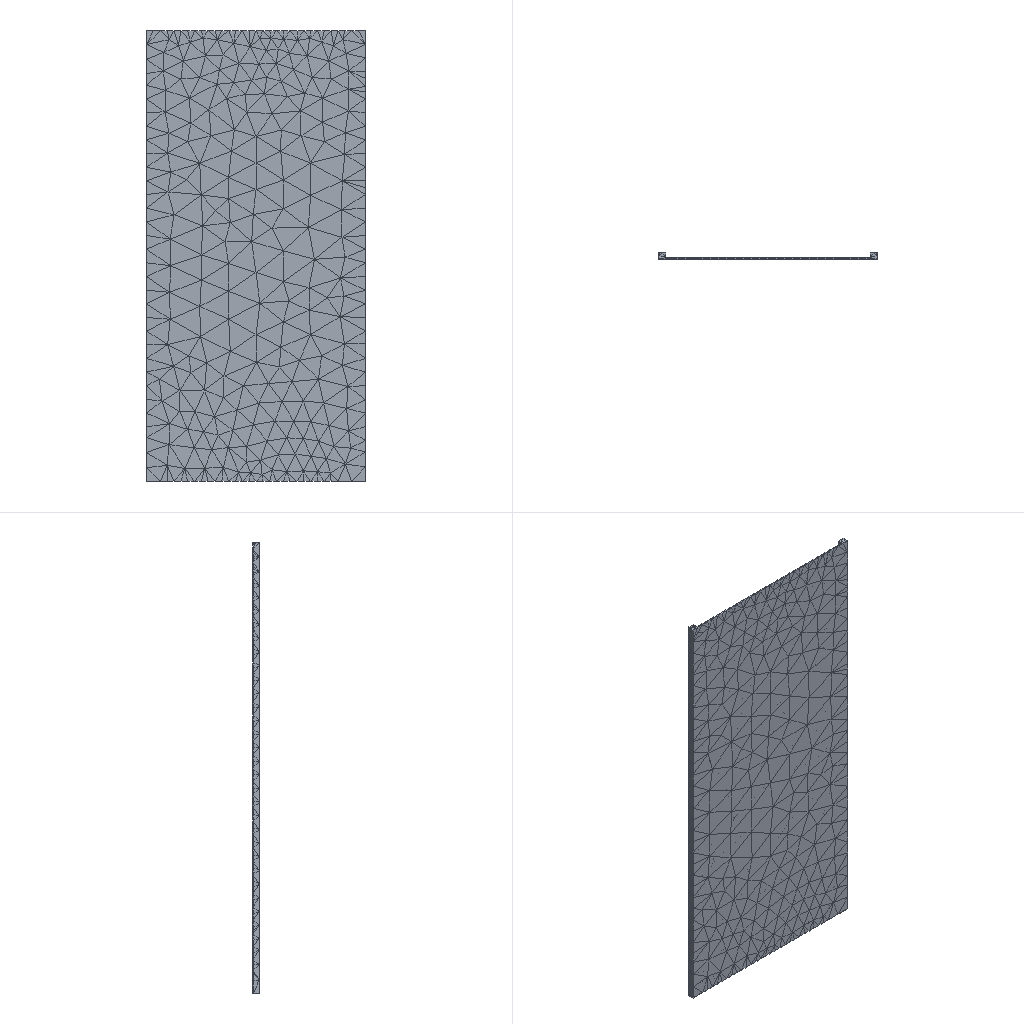Simulation study | ansys workbench
Ansys APDL input file, long lists of numbers shortened:
/batch
/config,noeldb,1     ! force off writing results to database
*get,_wallstrt,active,,time,wall
! ANSYS input file written by Workbench version 2022 R1
! File used for geometry attach: F:\ansys（分析文件汇总)\石材数控线距设备关键零部件分析\Master Assembly.STEP
/title,wbnew--____ (B5)
! ****** Begin Custom Load Command Snippet ******
/COM, ACT Extensions:
/COM,     LSDYNA, 2021.1
/COM,
! ****** End   Custom Load Command Snippet ******
*DIM,_wb_ProjectScratch_dir,string,248
_wb_ProjectScratch_dir(1) = 'C:\Users\Administrator\AppData\Local\Temp\WB_Administrator_1940_2\_ProjectScratch\Scr2DEB\'
*DIM,_wb_SolverFiles_dir,string,248
_wb_SolverFiles_dir(1) = 'C:\Users\Administrator\AppData\Local\Temp\WB_Administrator_1940_2\wbnew_files\dp0\SYS\MECH\'
*DIM,_wb_userfiles_dir,string,248
_wb_userfiles_dir(1) = 'C:\Users\Administrator\AppData\Local\Temp\WB_Administrator_1940_2\wbnew_files\user_files\'
/com,--- Data in consistent NMM units. See Solving Units in the help system for more information.
/units,MPA
/nopr
/wb,file,start              !  signify a WB generated input file
/prep7
! Turn off shape checking because checks already performed inside WB mesher.
! See help system for more information.
SHPP,OFF,,NOWARN
/nolist
etcon,set             ! allow ANSYS to choose best KEYOP's for 180x elements, resets any applicable keyopt to MAPDL defaults
/com,*********** Nodes for the whole assembly ***********
nblock,3,,450360
(1i9,3e20.9e3)
   128009     3.548597225E+02     4.820414370E+01    -3.842710506E+02
! (409418 more lines like these left out)
-1
/wb,elem,start            !  set before creation of elements
/com,*********** Elements for Body 1 "Ball Screw X Axis R14-5B1-FSW-189-271-0_008|Shaft-R14-5B1-FSW-189-271-0_008|NONE" ***********
et,1,187
eblock,19,solid,,1852
(19i9)
        1        1        1        1        0        0        0        0       10        0        1      264      596      682      593     2504     3611     2508     2503
! (3703 more lines like these left out)
-1
/com,*********** Elements for Body 2 "Ball Screw X Axis R14-5B1-FSW-189-271-0_008|R14-5B1-FSW|Cut-Extrude4" ***********
et,2,187
eblock,19,solid,,2828
(19i9)
        2        2        2        2        0        0        0        0       10        0     1853     4157     4736     4159     4734     7059     7076     7052     7058
! (5655 more lines like these left out)
-1
/com,*********** Elements for Body 3 "Ball Screw X Axis R14-5B1-FSW-189-271-0_008|WIPER-14-5|Revolve1" ***********
et,3,186
keyo,3,2,1          ! set full integration on SOLID186
eblock,19,solid,,12
(19i9)
        3        3        3        3        0        0        0        0       20        0     4681     9236     9246     9248     9249     9269     9268     9256     9255
! (23 more lines like these left out)
-1
/com,*********** Elements for Body 4 "Ball Screw X Axis R14-5B1-FSW-189-271-0_008|WIPER-14-5|Revolve1[2]" ***********
et,4,186
keyo,4,2,1          ! set full integration on SOLID186
eblock,19,solid,,12
(19i9)
        4        4        4        4        0        0        0        0       20        0     4693     9380     9390     9392     9393     9413     9412     9400     9399
! (23 more lines like these left out)
-1
/com,*********** Elements for Body 5 "HGW20 X Axis|Block Assembly^HGW20 X Axis|Block-HGW20CCZ0C|Cut-Extrude5" ***********
et,5,187
eblock,19,solid,,6973
(19i9)
        5        5        5        5        0        0        0        0       10        0     4705    10086    11155    11446    11445    15747    21059    15749    15748
! (13945 more lines like these left out)
-1
! (128 more sections like these left out)
/wb,elem,end               !  done creating elements
/com,*********** Send User Defined Coordinate System(s) ***********
csys,0
toffst,273.15,  ! Temperature offset from absolute zero
/com,*********** Set Reference Temperature ***********
tref,22.
/wb,mat,start              !  starting to send materials
/com,*********** Send Materials ***********
Temperature = 'TEMP' ! Temperature
MP,DENS,1,7.85e-09,	! tonne mm^-3
MP,ALPX,1,1.2e-05,	! C^-1
MP,C,1,434000000,	! mm^2 s^-2 C^-1
MP,KXX,1,60.5,	! tonne mm s^-3 C^-1
MP,RSVX,1,0.00017,	! ohm mm
MP,EX,1,200000,	! tonne s^-2 mm^-1
MP,NUXY,1,0.3,
MP,MURX,1,10000,
Temperature = 'TEMP' ! Temperature
MP,DENS,2,7.85e-09,	! tonne mm^-3
MP,ALPX,2,1.2e-05,	! C^-1
MP,C,2,434000000,	! mm^2 s^-2 C^-1
MP,KXX,2,60.5,	! tonne mm s^-3 C^-1
MP,RSVX,2,0.00017,	! ohm mm
MP,EX,2,200000,	! tonne s^-2 mm^-1
MP,NUXY,2,0.3,
MP,MURX,2,10000,
Temperature = 'TEMP' ! Temperature
MP,DENS,3,7.85e-09,	! tonne mm^-3
MP,ALPX,3,1.2e-05,	! C^-1
MP,C,3,434000000,	! mm^2 s^-2 C^-1
MP,KXX,3,60.5,	! tonne mm s^-3 C^-1
MP,RSVX,3,0.00017,	! ohm mm
MP,EX,3,200000,	! tonne s^-2 mm^-1
MP,NUXY,3,0.3,
MP,MURX,3,10000,
Temperature = 'TEMP' ! Temperature
MP,DENS,4,7.85e-09,	! tonne mm^-3
MP,ALPX,4,1.2e-05,	! C^-1
MP,C,4,434000000,	! mm^2 s^-2 C^-1
MP,KXX,4,60.5,	! tonne mm s^-3 C^-1
MP,RSVX,4,0.00017,	! ohm mm
MP,EX,4,200000,	! tonne s^-2 mm^-1
MP,NUXY,4,0.3,
MP,MURX,4,10000,
Temperature = 'TEMP' ! Temperature
MP,DENS,5,7.85e-09,	! tonne mm^-3
MP,ALPX,5,1.2e-05,	! C^-1
MP,C,5,434000000,	! mm^2 s^-2 C^-1
MP,KXX,5,60.5,	! tonne mm s^-3 C^-1
MP,RSVX,5,0.00017,	! ohm mm
MP,EX,5,200000,	! tonne s^-2 mm^-1
MP,NUXY,5,0.3,
MP,MURX,5,10000,
Temperature = 'TEMP' ! Temperature
MP,DENS,6,7.85e-09,	! tonne mm^-3
MP,ALPX,6,1.2e-05,	! C^-1
MP,C,6,434000000,	! mm^2 s^-2 C^-1
MP,KXX,6,60.5,	! tonne mm s^-3 C^-1
MP,RSVX,6,0.00017,	! ohm mm
MP,EX,6,200000,	! tonne s^-2 mm^-1
MP,NUXY,6,0.3,
MP,MURX,6,10000,
Temperature = 'TEMP' ! Temperature
MP,DENS,7,7.85e-09,	! tonne mm^-3
MP,ALPX,7,1.2e-05,	! C^-1
MP,C,7,434000000,	! mm^2 s^-2 C^-1
MP,KXX,7,60.5,	! tonne mm s^-3 C^-1
MP,RSVX,7,0.00017,	! ohm mm
MP,EX,7,200000,	! tonne s^-2 mm^-1
MP,NUXY,7,0.3,
MP,MURX,7,10000,
Temperature = 'TEMP' ! Temperature
MP,DENS,8,7.85e-09,	! tonne mm^-3
MP,ALPX,8,1.2e-05,	! C^-1
MP,C,8,434000000,	! mm^2 s^-2 C^-1
MP,KXX,8,60.5,	! tonne mm s^-3 C^-1
MP,RSVX,8,0.00017,	! ohm mm
MP,EX,8,200000,	! tonne s^-2 mm^-1
MP,NUXY,8,0.3,
MP,MURX,8,10000,
Temperature = 'TEMP' ! Temperature
MP,DENS,9,7.85e-09,	! tonne mm^-3
MP,ALPX,9,1.2e-05,	! C^-1
MP,C,9,434000000,	! mm^2 s^-2 C^-1
MP,KXX,9,60.5,	! tonne mm s^-3 C^-1
MP,RSVX,9,0.00017,	! ohm mm
MP,EX,9,200000,	! tonne s^-2 mm^-1
! (1118 more lines like these left out)
/wb,mat,end                !  done sending materials
!************************* Model Summary ********************
!Ball Screw X Axis R14-5B1-FSW-189-271-0_008|Shaft-R14-5B1-FSW-189-271-0_008|NONE,	结构钢,	matid,	1
!Ball Screw X Axis R14-5B1-FSW-189-271-0_008|R14-5B1-FSW|Cut-Extrude4,	结构钢,	matid,	2
!Ball Screw X Axis R14-5B1-FSW-189-271-0_008|WIPER-14-5|Revolve1,	结构钢,	matid,	3
! (132 more lines like these left out)
*get,_xmin,node,,mnloc,x
*get,_ymin,node,,mnloc,y
*get,_zmin,node,,mnloc,z
*get,_xmax,node,,mxloc,x
*get,_ymax,node,,mxloc,y
*get,_zmax,node,,mxloc,z
_ASMDIAG=(_xmax-_xmin)*(_xmax-_xmin)+(_ymax-_ymin)*(_ymax-_ymin)+(_zmax-_zmin)*(_zmax-_zmin)
_ASMDIAG=SQRT(_ASMDIAG)
/wb,contact,start          !  starting to send contact
/com,*********** Create Contact "接触区域" ***********
/com,            Real Constant Set For Above Contact Is 135 & 134
*set,tid,135
*set,cid,134
r,tid
r,cid
et,tid,170
et,cid,174
eblock,10,,,48
(15i9)
   324135      135      135      135        0       51       52      505      505     1067     1080      505     1073
! (47 more lines like these left out)
-1
eblock,10,,,48
(15i9)
   324183      134      134      134        0       51       52      505      505     1067     1080      505     1073
! (47 more lines like these left out)
-1
eblock,10,,,64
(15i9)
   324231      134      135      134        0     3979     4297     3975     3975     5779     5733     3975     5730
! (63 more lines like these left out)
-1
eblock,10,,,64
(15i9)
   324295      135      134      135        0     3979     4297     3975     3975     5779     5733     3975     5730
! (63 more lines like these left out)
-1
keyo,cid,8,2               ! auto create asymmetric contact (from Program Controlled setting)
keyo,cid,10,0              ! adjust contact stiffness each NR iteration (from Program Controlled setting)
keyo,cid,12,5              ! bonded always
keyo,cid,18,1              ! small sliding turned on by application
keyo,cid,2,0               ! augmented Lagrange (from Program Controlled setting)
keyo,cid,4,0               ! on Gauss point (from Program Controlled setting)
keyo,cid,9,1               ! ignore initial gaps/penetration
keyo,cid,7,0               ! No Prediction
rmod,tid,3,10.      ! FKN
rmod,tid,5,0.       ! ICONT
rmod,tid,6,0.       ! PINB
rmod,tid,10,0.      ! CNOF
rmod,tid,12,0.      ! FKT
rmod,tid,36,422     ! WB DSID
rmod,cid,3,10.      ! FKN
rmod,cid,5,0.       ! ICONT
rmod,cid,6,0.       ! PINB
rmod,cid,10,0.      ! CNOF
rmod,cid,12,0.      ! FKT
rmod,cid,36,422     ! WB DSID
/com,*********** Create Contact "接触区域 2" ***********
/com,            Real Constant Set For Above Contact Is 137 & 136
*set,tid,137
*set,cid,136
r,tid
r,cid
et,tid,170
et,cid,174
eblock,10,,,30
(15i9)
   324359      137      137      137        0       53       54      507      507     1084     1097      507     1090
! (29 more lines like these left out)
-1
eblock,10,,,30
(15i9)
   324389      136      136      136        0       53       54      507      507     1084     1097      507     1090
! (29 more lines like these left out)
-1
eblock,10,,,12
(15i9)
   324419      136      137      136        0     9253     9231     9274     9261     9281     9282     9353     9337
! (11 more lines like these left out)
-1
eblock,10,,,12
(15i9)
   324431      137      136      137        0     9253     9231     9274     9261     9281     9282     9353     9337
! (11 more lines like these left out)
-1
keyo,cid,8,2               ! auto create asymmetric contact (from Program Controlled setting)
keyo,cid,10,0              ! adjust contact stiffness each NR iteration (from Program Controlled setting)
keyo,cid,12,5              ! bonded always
keyo,cid,18,1              ! small sliding turned on by application
keyo,cid,2,0               ! augmented Lagrange (from Program Controlled setting)
keyo,cid,4,0               ! on Gauss point (from Program Controlled setting)
keyo,cid,9,1               ! ignore initial gaps/penetration
keyo,cid,7,0               ! No Prediction
rmod,tid,3,10.      ! FKN
rmod,tid,5,0.       ! ICONT
rmod,tid,6,0.       ! PINB
rmod,tid,10,0.      ! CNOF
rmod,tid,12,0.      ! FKT
rmod,tid,36,425     ! WB DSID
rmod,cid,3,10.      ! FKN
rmod,cid,5,0.       ! ICONT
rmod,cid,6,0.       ! PINB
rmod,cid,10,0.      ! CNOF
rmod,cid,12,0.      ! FKT
rmod,cid,36,425     ! WB DSID
/com,*********** Create Contact "接触区域 3" ***********
/com,            Real Constant Set For Above Contact Is 139 & 138
*set,tid,139
*set,cid,138
r,tid
r,cid
et,tid,170
et,cid,174
eblock,10,,,24
(15i9)
   324443      139      139      139        0       51       52      505      505     1067     1080      505     1073
! (23 more lines like these left out)
-1
eblock,10,,,24
(15i9)
   324467      138      138      138        0       51       52      505      505     1067     1080      505     1073
! (23 more lines like these left out)
-1
eblock,10,,,12
(15i9)
   324491      138      139      138        0     9392     9393     9399     9400     9470     9473     9483     9471
! (11 more lines like these left out)
-1
eblock,10,,,12
(15i9)
   324503      139      138      139        0     9392     9393     9399     9400     9470     9473     9483     9471
! (11 more lines like these left out)
-1
keyo,cid,8,2               ! auto create asymmetric contact (from Program Controlled setting)
keyo,cid,10,0              ! adjust contact stiffness each NR iteration (from Program Controlled setting)
keyo,cid,12,5              ! bonded always
keyo,cid,18,1              ! small sliding turned on by application
keyo,cid,2,0               ! augmented Lagrange (from Program Controlled setting)
keyo,cid,4,0               ! on Gauss point (from Program Controlled setting)
keyo,cid,9,1               ! ignore initial gaps/penetration
keyo,cid,7,0               ! No Prediction
rmod,tid,3,10.      ! FKN
rmod,tid,5,0.       ! ICONT
rmod,tid,6,0.       ! PINB
rmod,tid,10,0.      ! CNOF
rmod,tid,12,0.      ! FKT
rmod,tid,36,428     ! WB DSID
rmod,cid,3,10.      ! FKN
rmod,cid,5,0.       ! ICONT
rmod,cid,6,0.       ! PINB
rmod,cid,10,0.      ! CNOF
rmod,cid,12,0.      ! FKT
rmod,cid,36,428     ! WB DSID
/com,*********** Create Contact "接触区域 4" ***********
/com,            Real Constant Set For Above Contact Is 141 & 140
*set,tid,141
*set,cid,140
r,tid
r,cid
et,tid,170
et,cid,174
eblock,10,,,30
(15i9)
   324515      141      141      141        0       15       18       13       13      784      774       13      773
! (29 more lines like these left out)
-1
eblock,10,,,30
(15i9)
   324545      140      140      140        0       15       18       13       13      784      774       13      773
! (29 more lines like these left out)
-1
eblock,10,,,220
(15i9)
   324575      140      141      140        0   381566   381565   381678   381678   382469   382471   381678   382476
! (219 more lines like these left out)
-1
eblock,10,,,220
(15i9)
   324795      141      140      141        0   381566   381565   381678   381678   382469   382471   381678   382476
! (219 more lines like these left out)
-1
keyo,cid,8,2               ! auto create asymmetric contact (from Program Controlled setting)
keyo,cid,10,0              ! adjust contact stiffness each NR iteration (from Program Controlled setting)
keyo,cid,12,5              ! bonded always
keyo,cid,18,1              ! small sliding turned on by application
keyo,cid,2,0               ! augmented Lagrange (from Program Controlled setting)
keyo,cid,4,0               ! on Gauss point (from Program Controlled setting)
keyo,cid,9,1               ! ignore initial gaps/penetration
keyo,cid,7,0               ! No Prediction
rmod,tid,3,10.      ! FKN
rmod,tid,5,0.       ! ICONT
rmod,tid,6,0.       ! PINB
rmod,tid,10,0.      ! CNOF
rmod,tid,12,0.      ! FKT
rmod,tid,36,431     ! WB DSID
rmod,cid,3,10.      ! FKN
rmod,cid,5,0.       ! ICONT
rmod,cid,6,0.       ! PINB
rmod,cid,10,0.      ! CNOF
rmod,cid,12,0.      ! FKT
rmod,cid,36,431     ! WB DSID
/com,*********** Create Contact "接触区域 5" ***********
/com,            Real Constant Set For Above Contact Is 143 & 142
*set,tid,143
*set,cid,142
r,tid
r,cid
et,tid,170
et,cid,174
eblock,10,,,26
(15i9)
   325015      143      143      143        0      330      172      605      605     1976     1979      605     2735
! (25 more lines like these left out)
-1
eblock,10,,,26
(15i9)
   325041      142      142      142        0      330      172      605      605     1976     1979      605     2735
! (25 more lines like these left out)
-1
eblock,10,,,220
(15i9)
   325067      142      143      142        0   387692   387691   387804   387804   388595   388597   387804   388602
! (219 more lines like these left out)
-1
eblock,10,,,220
(15i9)
   325287      143      142      143        0   387692   387691   387804   387804   388595   388597   387804   388602
! (219 more lines like these left out)
-1
keyo,cid,8,2               ! auto create asymmetric contact (from Program Controlled setting)
keyo,cid,10,0              ! adjust contact stiffness each NR iteration (from Program Controlled setting)
keyo,cid,12,5              ! bonded always
keyo,cid,18,1              ! small sliding turned on by application
keyo,cid,2,0               ! augmented Lagrange (from Program Controlled setting)
keyo,cid,4,0               ! on Gauss point (from Program Controlled setting)
keyo,cid,9,1               ! ignore initial gaps/penetration
keyo,cid,7,0               ! No Prediction
rmod,tid,3,10.      ! FKN
rmod,tid,5,0.       ! ICONT
rmod,tid,6,0.       ! PINB
rmod,tid,10,0.      ! CNOF
rmod,tid,12,0.      ! FKT
rmod,tid,36,434     ! WB DSID
rmod,cid,3,10.      ! FKN
rmod,cid,5,0.       ! ICONT
rmod,cid,6,0.       ! PINB
rmod,cid,10,0.      ! CNOF
rmod,cid,12,0.      ! FKT
rmod,cid,36,434     ! WB DSID
! (365 more sections like these left out)
/wb,contact,end            !  done creating contacts
/golist
/wb,load,start             !  starting to send loads
/com,*********** Fixed Supports ***********
CMBLOCK,_FIXEDSU,NODE,   208462
(8i10)
         1         2         3         4         5         6         7         8
! (26057 more lines like these left out)
cmsel,s,_FIXEDSU
d,all,all
nsel,all
/com,*********** Define Force Using Surface Effect Elements ***********
local,12,0,0.,0.,0.,0.,0.,0.
csys,0
et,874,154
eblock,10,,,4919
(15i9)
   442965      874      874      874       12   392433   391384   392435   392434   395655   395656   397819   397817
! (4918 more lines like these left out)
-1
esel,s,type,,874
keyop,874,2,1                ! Apply load in local coordinate system
keyop,874,7,1                ! Use original area so load is constant in large deformation
esel,all
/gst,on,on
fini
*get,_numnode,node,0,count
*get,_numelem,elem,0,count
*get, _MAXELEMNUM, elem, 0, NUM, MAX
*get, _MAXNODENUM, node, 0, NUM, MAX
*get, _MAXELEMTYPE, etyp, 0, NUM, MAX
*get, _MAXREALCONST, real, 0, NUM, MAX
/go
/wb,load,end               !  done creating loads
/com,--- Number of total nodes = %_numnode%
/com,--- Number of contact elements = 123749
/com,--- Number of spring elements = 0
/com,--- Number of bearing elements = 0
/com,--- Number of solid elements = 213356
/com,--- Number of condensed parts = 0
/com,--- Number of total elements = %_numelem%
*get,_wallbsol,active,,time,wall
/com,****************************************************************************
/com,*************************    SOLUTION       ********************************
/com,****************************************************************************
/solu
antype,0                   ! static analysis
_thickRatio=0.271   ! Ratio of thick parts in the model
eqsl,sparse,,,,,1
cntr,print,1               ! print out contact info and also make no initial contact an error
cntr,out,yes               ! write contact output to file.cmn due to many contact pairs present
dmpoption,emat,no             ! Don't combine emat file for DANSYS
dmpoption,esav,no             ! Don't combine esav file for DANSYS
nldiag,cont,iter           ! print out contact info each equilibrium iteration
rescontrol,,none                 ! Do not keep any restart files
/com,****************************************************
/com,******************* SOLVE FOR LS 1 OF 1 ****************
esel,s,type,,874
nsle
sfe,all,1,pres,1,8.35430170226117e-015
sfe,all,2,pres,1,-2.785
sfe,all,3,pres,1,0.
nsel,all
esel,all
/nopr
/gopr
nsub,1,1,1
time,1.
outres,erase
outres,all,none
outres,nsol,all,
outres,rsol,all
outres,eangl,all
outres,etmp,all
outres,veng,all
outres,strs,all,
outres,epel,all,
outres,eppl,all,
outres,cont,all,
! *********** WB SOLVE COMMAND ***********
! check interactive state
*get,ANSINTER_,active,,int
*if,ANSINTER_,ne,0,then
/eof
*endif
solve
/com *************** Write FE CONNECTORS *********
CEWRITE,file,ce,,INTE
/com,****************************************************
/com,*************** FINISHED SOLVE FOR LS 1 *************
*get,_wallasol,active,,time,wall
/nopr
*get,_numnode,node,0,count
*get,_numelem,elem,0,count
*get, _MAXELEMNUM, elem, 0, NUM, MAX
*get, _MAXNODENUM, node, 0, NUM, MAX,,,INTERNAL
*get, _MAXELEMTYPE, etyp, 0, NUM, MAX
*get, _MAXREALCONST, real, 0, NUM, MAX
/gopr
/post1
xmlo,ENCODING,ISO-8859-1
xmlo,parm
/xml,parm,xml
fini
/gopr
*get,_walldone,active,,time,wall
_preptime=(_wallbsol-_wallstrt)*3600
_solvtime=(_wallasol-_wallbsol)*3600
_posttime=(_walldone-_wallasol)*3600
_totaltim=(_walldone-_wallstrt)*3600
*get,_dlbratio,active,0,solu,dlbr
*get,_combtime,active,0,solu,comb
*get,_ssmode,active,0,solu,ssmm
*get,_ndofs,active,0,solu,ndof
*get,_sol_end_time,active,0,set,time
*if,_sol_end_time,eq,1.,then
/fclean				!clean distributed files
*endif
/com,--- Total number of nodes = %_numnode%
/com,--- Total number of elements = %_numelem%
/com,--- Element load balance ratio = %_dlbratio%
/com,--- Time to combine distributed files = %_combtime%
/com,--- Sparse memory mode = %_ssmode%
/com,--- Number of DOF = %_ndofs%
/wb,file,end               ! done with WB generated input